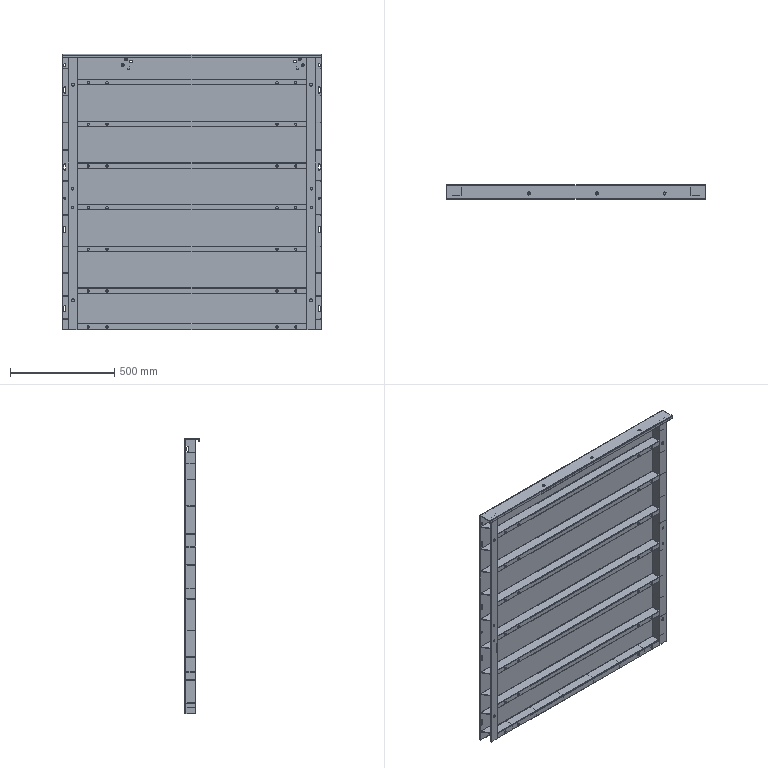Part | 45 solids | 962 faces | box 1240 x 70 x 1320 mm | volume 8173889 mm3 | plane 612 | cylinder 308 | cone 42 | commonest cylinder face diameters 11 x112 10 x70 0.4 x22 6.917 x14 10.45 x14 10.5 x14